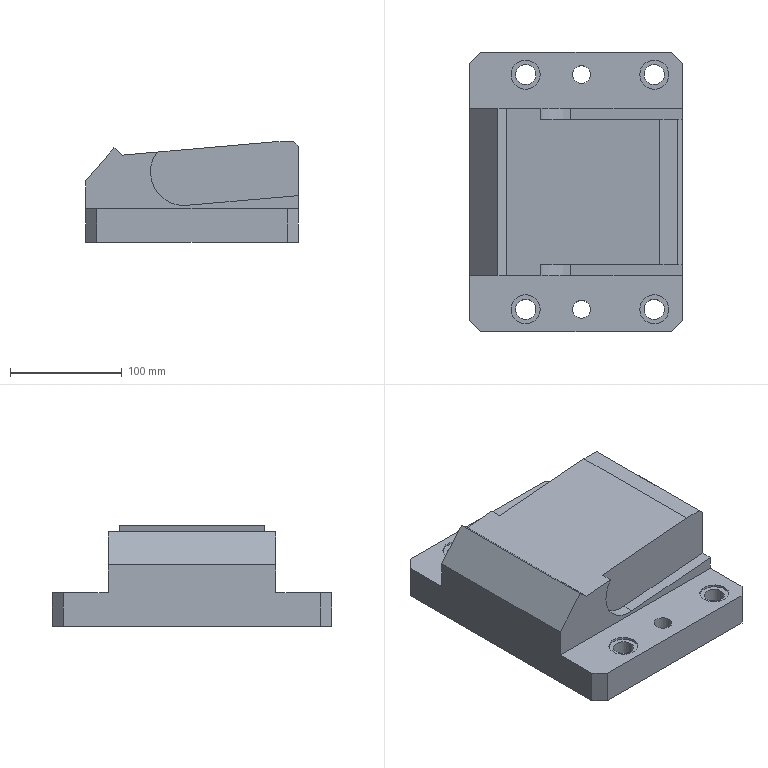Part | NX | features solid 2 | 1 solid | 51 faces | box 190 x 250 x 90 mm | volume 2700369 mm3 | plane 35 | cylinder 16 | commonest cylinder face diameters 18 x4 20 x4 26 x4 16 x2 60 x2
STEP:
#1=CARTESIAN_POINT('',(1060.,115.,-248.228));
#2=VERTEX_POINT('',#1);
#3=CARTESIAN_POINT('',(1060.,115.,-204.));
#4=VERTEX_POINT('',#3);
#5=CARTESIAN_POINT('',(1060.,115.,-218.327));
#6=DIRECTION('',(0.,0.,1.));
#7=VECTOR('',#6,1000.);
#8=LINE('',#5,#7);
#9=EDGE_CURVE('',#2,#4,#8,.T.);
#10=ORIENTED_EDGE('',*,*,#9,.F.);
#11=CARTESIAN_POINT('',(1060.,105.,-248.228));
#12=VERTEX_POINT('',#11);
#13=CARTESIAN_POINT('',(1060.,180.,-248.228));
#14=DIRECTION('',(0.,-1.,0.));
#15=VECTOR('',#14,1000.);
#16=LINE('',#13,#15);
#17=EDGE_CURVE('',#12,#2,#16,.F.);
#18=ORIENTED_EDGE('',*,*,#17,.F.);
#19=CARTESIAN_POINT('',(1060.,105.,-260.));
#20=VERTEX_POINT('',#19);
#21=CARTESIAN_POINT('',(1060.,105.,-200.));
#22=DIRECTION('',(0.,0.,-1.));
#23=VECTOR('',#22,1000.);
#24=LINE('',#21,#23);
#25=EDGE_CURVE('',#12,#20,#24,.T.);
#26=ORIENTED_EDGE('',*,*,#25,.T.);
#27=CARTESIAN_POINT('',(1060.,65.,-260.));
#28=VERTEX_POINT('',#27);
#29=CARTESIAN_POINT('',(1060.,305.,-260.));
#30=DIRECTION('',(0.,-1.,0.));
#31=VECTOR('',#30,1000.);
#32=LINE('',#29,#31);
#33=EDGE_CURVE('',#20,#28,#32,.T.);
#34=ORIENTED_EDGE('',*,*,#33,.T.);
#35=CARTESIAN_POINT('',(1060.,65.,-290.));
#36=VERTEX_POINT('',#35);
#37=CARTESIAN_POINT('',(1060.,65.,-260.));
#38=DIRECTION('',(0.,0.,1.));
#39=VECTOR('',#38,1000.);
#40=LINE('',#37,#39);
#41=EDGE_CURVE('',#36,#28,#40,.T.);
#42=ORIENTED_EDGE('',*,*,#41,.F.);
#43=CARTESIAN_POINT('',(1060.,295.,-290.));
#44=VERTEX_POINT('',#43);
#45=CARTESIAN_POINT('',(1060.,305.,-290.));
#46=DIRECTION('',(0.,-1.,0.));
#47=VECTOR('',#46,1000.);
#48=LINE('',#45,#47);
#49=EDGE_CURVE('',#44,#36,#48,.T.);
#50=ORIENTED_EDGE('',*,*,#49,.F.);
#51=CARTESIAN_POINT('',(1060.,295.,-260.));
#52=VERTEX_POINT('',#51);
#53=CARTESIAN_POINT('',(1060.,295.,-260.));
#54=DIRECTION('',(0.,0.,-1.));
#55=VECTOR('',#54,1000.);
#56=LINE('',#53,#55);
#57=EDGE_CURVE('',#52,#44,#56,.T.);
#58=ORIENTED_EDGE('',*,*,#57,.F.);
#59=CARTESIAN_POINT('',(1060.,255.,-260.));
#60=VERTEX_POINT('',#59);
#61=CARTESIAN_POINT('',(1060.,305.,-260.));
#62=DIRECTION('',(0.,-1.,0.));
#63=VECTOR('',#62,1000.);
#64=LINE('',#61,#63);
#65=EDGE_CURVE('',#52,#60,#64,.T.);
#66=ORIENTED_EDGE('',*,*,#65,.T.);
#67=CARTESIAN_POINT('',(1060.,255.,-248.228));
#68=VERTEX_POINT('',#67);
#69=CARTESIAN_POINT('',(1060.,255.,-200.));
#70=DIRECTION('',(0.,0.,-1.));
#71=VECTOR('',#70,1000.);
#72=LINE('',#69,#71);
#73=EDGE_CURVE('',#68,#60,#72,.T.);
#74=ORIENTED_EDGE('',*,*,#73,.F.);
#75=CARTESIAN_POINT('',(1060.,245.,-248.228));
#76=VERTEX_POINT('',#75);
#77=CARTESIAN_POINT('',(1060.,180.,-248.228));
#78=DIRECTION('',(0.,1.,0.));
#79=VECTOR('',#78,1000.);
#80=LINE('',#77,#79);
#81=EDGE_CURVE('',#68,#76,#80,.F.);
#82=ORIENTED_EDGE('',*,*,#81,.T.);
#83=CARTESIAN_POINT('',(1060.,245.,-204.));
#84=VERTEX_POINT('',#83);
#85=CARTESIAN_POINT('',(1060.,245.,-218.327));
#86=DIRECTION('',(0.,0.,1.));
#87=VECTOR('',#86,1000.);
#88=LINE('',#85,#87);
#89=EDGE_CURVE('',#76,#84,#88,.T.);
#90=ORIENTED_EDGE('',*,*,#89,.T.);
#91=CARTESIAN_POINT('',(1060.,305.,-204.));
#92=DIRECTION('',(0.,1.,0.));
#93=VECTOR('',#92,1000.);
#94=LINE('',#91,#93);
#95=EDGE_CURVE('',#4,#84,#94,.T.);
#96=ORIENTED_EDGE('',*,*,#95,.F.);
#97=EDGE_LOOP('',(#10,#18,#26,#34,#42,#50,#58,#66,#74,#82,#90,#96));
#98=FACE_BOUND('',#97,.T.);
#99=CARTESIAN_POINT('',(1060.,305.,-260.));
#100=DIRECTION('',(1.,0.,0.));
#101=DIRECTION('',(0.,-1.,0.));
#102=AXIS2_PLACEMENT_3D('',#99,#100,#101);
#103=PLANE('',#102);
#104=ADVANCED_FACE('',(#98),#103,.T.);
#105=CARTESIAN_POINT('',(933.612,245.,-209.308));
#106=VERTEX_POINT('',#105);
#107=CARTESIAN_POINT('',(933.612,255.,-209.308));
#108=VERTEX_POINT('',#107);
#109=CARTESIAN_POINT('',(933.612,250.,-209.308));
#110=DIRECTION('',(0.,1.,0.));
#111=VECTOR('',#110,1000.);
#112=LINE('',#109,#111);
#113=EDGE_CURVE('',#106,#108,#112,.T.);
#114=ORIENTED_EDGE('',*,*,#113,.T.);
#115=CARTESIAN_POINT('',(902.806,255.,-212.003));
#116=VERTEX_POINT('',#115);
#117=CARTESIAN_POINT('',(1040.,255.,-200.));
#118=DIRECTION('',(-0.9962,0.,-0.08716));
#119=VECTOR('',#118,1000.);
#120=LINE('',#117,#119);
#121=EDGE_CURVE('',#108,#116,#120,.T.);
#122=ORIENTED_EDGE('',*,*,#121,.T.);
#123=CARTESIAN_POINT('',(902.806,105.,-212.003));
#124=VERTEX_POINT('',#123);
#125=CARTESIAN_POINT('',(902.806,255.,-212.003));
#126=DIRECTION('',(0.,-1.,0.));
#127=VECTOR('',#126,1000.);
#128=LINE('',#125,#127);
#129=EDGE_CURVE('',#116,#124,#128,.T.);
#130=ORIENTED_EDGE('',*,*,#129,.T.);
#131=CARTESIAN_POINT('',(933.612,105.,-209.308));
#132=VERTEX_POINT('',#131);
#133=CARTESIAN_POINT('',(1040.,105.,-200.));
#134=DIRECTION('',(-0.9962,0.,-0.08716));
#135=VECTOR('',#134,1000.);
#136=LINE('',#133,#135);
#137=EDGE_CURVE('',#132,#124,#136,.T.);
#138=ORIENTED_EDGE('',*,*,#137,.F.);
#139=CARTESIAN_POINT('',(933.612,115.,-209.308));
#140=VERTEX_POINT('',#139);
#141=CARTESIAN_POINT('',(933.612,110.,-209.308));
#142=DIRECTION('',(0.,1.,0.));
#143=VECTOR('',#142,1000.);
#144=LINE('',#141,#143);
#145=EDGE_CURVE('',#132,#140,#144,.T.);
#146=ORIENTED_EDGE('',*,*,#145,.T.);
#147=CARTESIAN_POINT('',(1040.,115.,-200.));
#148=VERTEX_POINT('',#147);
#149=CARTESIAN_POINT('',(1040.,115.,-200.));
#150=DIRECTION('',(0.9962,0.,0.08716));
#151=VECTOR('',#150,1000.);
#152=LINE('',#149,#151);
#153=EDGE_CURVE('',#140,#148,#152,.T.);
#154=ORIENTED_EDGE('',*,*,#153,.T.);
#155=CARTESIAN_POINT('',(1040.,245.,-200.));
#156=VERTEX_POINT('',#155);
#157=CARTESIAN_POINT('',(1040.,255.,-200.));
#158=DIRECTION('',(0.,-1.,0.));
#159=VECTOR('',#158,1000.);
#160=LINE('',#157,#159);
#161=EDGE_CURVE('',#156,#148,#160,.T.);
#162=ORIENTED_EDGE('',*,*,#161,.F.);
#163=CARTESIAN_POINT('',(1040.,245.,-200.));
#164=DIRECTION('',(-0.9962,0.,-0.08716));
#165=VECTOR('',#164,1000.);
#166=LINE('',#163,#165);
#167=EDGE_CURVE('',#156,#106,#166,.T.);
#168=ORIENTED_EDGE('',*,*,#167,.T.);
#169=EDGE_LOOP('',(#114,#122,#130,#138,#146,#154,#162,#168));
#170=FACE_BOUND('',#169,.T.);
#171=CARTESIAN_POINT('',(1040.,255.,-200.));
#172=DIRECTION('',(0.08716,0.,-0.9962));
#173=DIRECTION('',(-0.9962,0.,-0.08716));
#174=AXIS2_PLACEMENT_3D('',#171,#172,#173);
#175=PLANE('',#174);
#176=ADVANCED_FACE('',(#170),#175,.F.);
#177=CARTESIAN_POINT('',(1056.,245.,-200.));
#178=VERTEX_POINT('',#177);
#179=CARTESIAN_POINT('',(1040.,245.,-200.));
#180=DIRECTION('',(1.,0.,0.));
#181=VECTOR('',#180,1000.);
#182=LINE('',#179,#181);
#183=EDGE_CURVE('',#156,#178,#182,.T.);
#184=ORIENTED_EDGE('',*,*,#183,.F.);
#185=ORIENTED_EDGE('',*,*,#161,.T.);
#186=CARTESIAN_POINT('',(1056.,115.,-200.));
#187=VERTEX_POINT('',#186);
#188=CARTESIAN_POINT('',(1040.,115.,-200.));
#189=DIRECTION('',(-1.,0.,0.));
#190=VECTOR('',#189,1000.);
#191=LINE('',#188,#190);
#192=EDGE_CURVE('',#187,#148,#191,.T.);
#193=ORIENTED_EDGE('',*,*,#192,.F.);
#194=CARTESIAN_POINT('',(1056.,255.,-200.));
#195=DIRECTION('',(0.,-1.,0.));
#196=VECTOR('',#195,1000.);
#197=LINE('',#194,#196);
#198=EDGE_CURVE('',#178,#187,#197,.T.);
#199=ORIENTED_EDGE('',*,*,#198,.F.);
#200=EDGE_LOOP('',(#184,#185,#193,#199));
#201=FACE_BOUND('',#200,.T.);
#202=CARTESIAN_POINT('',(1040.,255.,-200.));
#203=DIRECTION('',(0.,0.,1.));
#204=DIRECTION('',(0.,-1.,0.));
#205=AXIS2_PLACEMENT_3D('',#202,#203,#204);
#206=PLANE('',#205);
#207=ADVANCED_FACE('',(#201),#206,.T.);
#208=ORIENTED_EDGE('',*,*,#73,.T.);
#209=CARTESIAN_POINT('',(870.,255.,-260.));
#210=VERTEX_POINT('',#209);
#211=CARTESIAN_POINT('',(870.,255.,-260.));
#212=DIRECTION('',(1.,0.,0.));
#213=VECTOR('',#212,1000.);
#214=LINE('',#211,#213);
#215=EDGE_CURVE('',#210,#60,#214,.T.);
#216=ORIENTED_EDGE('',*,*,#215,.F.);
#217=CARTESIAN_POINT('',(870.,255.,-235.));
#218=VERTEX_POINT('',#217);
#219=CARTESIAN_POINT('',(870.,255.,-235.));
#220=DIRECTION('',(0.,0.,-1.));
#221=VECTOR('',#220,1000.);
#222=LINE('',#219,#221);
#223=EDGE_CURVE('',#218,#210,#222,.T.);
#224=ORIENTED_EDGE('',*,*,#223,.F.);
#225=CARTESIAN_POINT('',(895.204,255.,-205.506));
#226=VERTEX_POINT('',#225);
#227=CARTESIAN_POINT('',(870.,255.,-235.));
#228=DIRECTION('',(0.6497,0.,0.7602));
#229=VECTOR('',#228,1000.);
#230=LINE('',#227,#229);
#231=EDGE_CURVE('',#218,#226,#230,.T.);
#232=ORIENTED_EDGE('',*,*,#231,.T.);
#233=CARTESIAN_POINT('',(895.204,255.,-205.506));
#234=DIRECTION('',(0.7602,0.,-0.6497));
#235=VECTOR('',#234,1000.);
#236=LINE('',#233,#235);
#237=EDGE_CURVE('',#226,#116,#236,.T.);
#238=ORIENTED_EDGE('',*,*,#237,.T.);
#239=ORIENTED_EDGE('',*,*,#121,.F.);
#240=CARTESIAN_POINT('',(960.414,255.,-256.94));
#241=VERTEX_POINT('',#240);
#242=CARTESIAN_POINT('',(957.8,255.,-227.054));
#243=DIRECTION('',(0.,-1.,0.));
#244=DIRECTION('',(1.,0.,0.));
#245=AXIS2_PLACEMENT_3D('',#242,#243,#244);
#246=CIRCLE('',#245,30.);
#247=EDGE_CURVE('',#241,#108,#246,.F.);
#248=ORIENTED_EDGE('',*,*,#247,.F.);
#249=CARTESIAN_POINT('',(1060.,255.,-248.228));
#250=DIRECTION('',(-0.9962,0.,-0.08716));
#251=VECTOR('',#250,1000.);
#252=LINE('',#249,#251);
#253=EDGE_CURVE('',#68,#241,#252,.T.);
#254=ORIENTED_EDGE('',*,*,#253,.F.);
#255=EDGE_LOOP('',(#208,#216,#224,#232,#238,#239,#248,#254));
#256=FACE_BOUND('',#255,.T.);
#257=CARTESIAN_POINT('',(870.,255.,-214.873));
#258=DIRECTION('',(0.,1.,0.));
#259=DIRECTION('',(1.,0.,0.));
#260=AXIS2_PLACEMENT_3D('',#257,#258,#259);
#261=PLANE('',#260);
#262=ADVANCED_FACE('',(#256),#261,.T.);
#263=CARTESIAN_POINT('',(960.414,105.,-256.94));
#264=VERTEX_POINT('',#263);
#265=CARTESIAN_POINT('',(1060.,105.,-248.228));
#266=DIRECTION('',(-0.9962,0.,-0.08716));
#267=VECTOR('',#266,1000.);
#268=LINE('',#265,#267);
#269=EDGE_CURVE('',#12,#264,#268,.T.);
#270=ORIENTED_EDGE('',*,*,#269,.T.);
#271=CARTESIAN_POINT('',(957.8,105.,-227.054));
#272=DIRECTION('',(0.,-1.,0.));
#273=DIRECTION('',(1.,0.,0.));
#274=AXIS2_PLACEMENT_3D('',#271,#272,#273);
#275=CIRCLE('',#274,30.);
#276=EDGE_CURVE('',#132,#264,#275,.T.);
#277=ORIENTED_EDGE('',*,*,#276,.F.);
#278=ORIENTED_EDGE('',*,*,#137,.T.);
#279=CARTESIAN_POINT('',(895.204,105.,-205.506));
#280=VERTEX_POINT('',#279);
#281=CARTESIAN_POINT('',(895.204,105.,-205.506));
#282=DIRECTION('',(0.7602,0.,-0.6497));
#283=VECTOR('',#282,1000.);
#284=LINE('',#281,#283);
#285=EDGE_CURVE('',#280,#124,#284,.T.);
#286=ORIENTED_EDGE('',*,*,#285,.F.);
#287=CARTESIAN_POINT('',(870.,105.,-235.));
#288=VERTEX_POINT('',#287);
#289=CARTESIAN_POINT('',(870.,105.,-235.));
#290=DIRECTION('',(0.6497,0.,0.7602));
#291=VECTOR('',#290,1000.);
#292=LINE('',#289,#291);
#293=EDGE_CURVE('',#288,#280,#292,.T.);
#294=ORIENTED_EDGE('',*,*,#293,.F.);
#295=CARTESIAN_POINT('',(870.,105.,-260.));
#296=VERTEX_POINT('',#295);
#297=CARTESIAN_POINT('',(870.,105.,-235.));
#298=DIRECTION('',(0.,0.,-1.));
#299=VECTOR('',#298,1000.);
#300=LINE('',#297,#299);
#301=EDGE_CURVE('',#288,#296,#300,.T.);
#302=ORIENTED_EDGE('',*,*,#301,.T.);
#303=CARTESIAN_POINT('',(870.,105.,-260.));
#304=DIRECTION('',(1.,0.,0.));
#305=VECTOR('',#304,1000.);
#306=LINE('',#303,#305);
#307=EDGE_CURVE('',#296,#20,#306,.T.);
#308=ORIENTED_EDGE('',*,*,#307,.T.);
#309=ORIENTED_EDGE('',*,*,#25,.F.);
#310=EDGE_LOOP('',(#270,#277,#278,#286,#294,#302,#308,#309));
#311=FACE_BOUND('',#310,.T.);
#312=CARTESIAN_POINT('',(870.,105.,-214.873));
#313=DIRECTION('',(0.,1.,0.));
#314=DIRECTION('',(1.,0.,0.));
#315=AXIS2_PLACEMENT_3D('',#312,#313,#314);
#316=PLANE('',#315);
#317=ADVANCED_FACE('',(#311),#316,.F.);
#318=CARTESIAN_POINT('',(978.,75.,-260.));
#319=VERTEX_POINT('',#318);
#320=CARTESIAN_POINT('',(970.,75.,-260.));
#321=DIRECTION('',(0.,0.,1.));
#322=DIRECTION('',(1.,0.,0.));
#323=AXIS2_PLACEMENT_3D('',#320,#321,#322);
#324=CIRCLE('',#323,8.);
#325=EDGE_CURVE('',#319,#319,#324,.T.);
#326=ORIENTED_EDGE('',*,*,#325,.F.);
#327=EDGE_LOOP('',(#326));
#328=FACE_BOUND('',#327,.T.);
#329=CARTESIAN_POINT('',(907.,75.,-260.));
#330=VERTEX_POINT('',#329);
#331=CARTESIAN_POINT('',(920.,75.,-260.));
#332=DIRECTION('',(0.,0.,-1.));
#333=DIRECTION('',(-1.,0.,0.));
#334=AXIS2_PLACEMENT_3D('',#331,#332,#333);
#335=CIRCLE('',#334,13.);
#336=EDGE_CURVE('',#330,#330,#335,.F.);
#337=ORIENTED_EDGE('',*,*,#336,.F.);
#338=EDGE_LOOP('',(#337));
#339=FACE_BOUND('',#338,.T.);
#340=CARTESIAN_POINT('',(1022.,75.,-260.));
#341=VERTEX_POINT('',#340);
#342=CARTESIAN_POINT('',(1035.,75.,-260.));
#343=DIRECTION('',(0.,0.,-1.));
#344=DIRECTION('',(-1.,0.,0.));
#345=AXIS2_PLACEMENT_3D('',#342,#343,#344);
#346=CIRCLE('',#345,13.);
#347=EDGE_CURVE('',#341,#341,#346,.F.);
#348=ORIENTED_EDGE('',*,*,#347,.F.);
#349=EDGE_LOOP('',(#348));
#350=FACE_BOUND('',#349,.T.);
#351=CARTESIAN_POINT('',(880.,55.,-260.));
#352=VERTEX_POINT('',#351);
#353=CARTESIAN_POINT('',(1050.,55.,-260.));
#354=VERTEX_POINT('',#353);
#355=CARTESIAN_POINT('',(870.,55.,-260.));
#356=DIRECTION('',(1.,0.,0.));
#357=VECTOR('',#356,1000.);
#358=LINE('',#355,#357);
#359=EDGE_CURVE('',#352,#354,#358,.T.);
#360=ORIENTED_EDGE('',*,*,#359,.T.);
#361=CARTESIAN_POINT('',(1085.,90.,-260.));
#362=DIRECTION('',(-0.7071,-0.7071,0.));
#363=VECTOR('',#362,1000.);
#364=LINE('',#361,#363);
#365=EDGE_CURVE('',#28,#354,#364,.T.);
#366=ORIENTED_EDGE('',*,*,#365,.F.);
#367=ORIENTED_EDGE('',*,*,#33,.F.);
#368=ORIENTED_EDGE('',*,*,#307,.F.);
#369=CARTESIAN_POINT('',(870.,65.,-260.));
#370=VERTEX_POINT('',#369);
#371=CARTESIAN_POINT('',(870.,305.,-260.));
#372=DIRECTION('',(0.,-1.,0.));
#373=VECTOR('',#372,1000.);
#374=LINE('',#371,#373);
#375=EDGE_CURVE('',#296,#370,#374,.T.);
#376=ORIENTED_EDGE('',*,*,#375,.T.);
#377=CARTESIAN_POINT('',(750.,185.,-260.));
#378=DIRECTION('',(0.7071,-0.7071,0.));
#379=VECTOR('',#378,1000.);
#380=LINE('',#377,#379);
#381=EDGE_CURVE('',#352,#370,#380,.F.);
#382=ORIENTED_EDGE('',*,*,#381,.F.);
#383=EDGE_LOOP('',(#360,#366,#367,#368,#376,#382));
#384=FACE_BOUND('',#383,.T.);
#385=CARTESIAN_POINT('',(870.,305.,-260.));
#386=DIRECTION('',(0.,0.,1.));
#387=DIRECTION('',(1.,0.,0.));
#388=AXIS2_PLACEMENT_3D('',#385,#386,#387);
#389=PLANE('',#388);
#390=ADVANCED_FACE('',(#328,#339,#350,#384),#389,.T.);
#391=CARTESIAN_POINT('',(870.,295.,-290.));
#392=VERTEX_POINT('',#391);
#393=CARTESIAN_POINT('',(870.,65.,-290.));
#394=VERTEX_POINT('',#393);
#395=CARTESIAN_POINT('',(870.,305.,-290.));
#396=DIRECTION('',(0.,-1.,0.));
#397=VECTOR('',#396,1000.);
#398=LINE('',#395,#397);
#399=EDGE_CURVE('',#392,#394,#398,.T.);
#400=ORIENTED_EDGE('',*,*,#399,.T.);
#401=CARTESIAN_POINT('',(870.,65.,-260.));
#402=DIRECTION('',(0.,0.,-1.));
#403=VECTOR('',#402,1000.);
#404=LINE('',#401,#403);
#405=EDGE_CURVE('',#370,#394,#404,.T.);
#406=ORIENTED_EDGE('',*,*,#405,.F.);
#407=ORIENTED_EDGE('',*,*,#375,.F.);
#408=ORIENTED_EDGE('',*,*,#301,.F.);
#409=CARTESIAN_POINT('',(870.,255.,-235.));
#410=DIRECTION('',(0.,-1.,0.));
#411=VECTOR('',#410,1000.);
#412=LINE('',#409,#411);
#413=EDGE_CURVE('',#218,#288,#412,.T.);
#414=ORIENTED_EDGE('',*,*,#413,.F.);
#415=ORIENTED_EDGE('',*,*,#223,.T.);
#416=CARTESIAN_POINT('',(870.,295.,-260.));
#417=VERTEX_POINT('',#416);
#418=CARTESIAN_POINT('',(870.,305.,-260.));
#419=DIRECTION('',(0.,-1.,0.));
#420=VECTOR('',#419,1000.);
#421=LINE('',#418,#420);
#422=EDGE_CURVE('',#417,#210,#421,.T.);
#423=ORIENTED_EDGE('',*,*,#422,.F.);
#424=CARTESIAN_POINT('',(870.,295.,-260.));
#425=DIRECTION('',(0.,0.,1.));
#426=VECTOR('',#425,1000.);
#427=LINE('',#424,#426);
#428=EDGE_CURVE('',#392,#417,#427,.T.);
#429=ORIENTED_EDGE('',*,*,#428,.F.);
#430=EDGE_LOOP('',(#400,#406,#407,#408,#414,#415,#423,#429));
#431=FACE_BOUND('',#430,.T.);
#432=CARTESIAN_POINT('',(870.,305.,-260.));
#433=DIRECTION('',(1.,0.,0.));
#434=DIRECTION('',(0.,-1.,0.));
#435=AXIS2_PLACEMENT_3D('',#432,#433,#434);
#436=PLANE('',#435);
#437=ADVANCED_FACE('',(#431),#436,.F.);
#438=CARTESIAN_POINT('',(978.,75.,-290.));
#439=VERTEX_POINT('',#438);
#440=CARTESIAN_POINT('',(970.,75.,-290.));
#441=DIRECTION('',(0.,0.,1.));
#442=DIRECTION('',(1.,0.,0.));
#443=AXIS2_PLACEMENT_3D('',#440,#441,#442);
#444=CIRCLE('',#443,8.);
#445=EDGE_CURVE('',#439,#439,#444,.T.);
#446=ORIENTED_EDGE('',*,*,#445,.T.);
#447=EDGE_LOOP('',(#446));
#448=FACE_BOUND('',#447,.T.);
#449=CARTESIAN_POINT('',(978.,285.,-290.));
#450=VERTEX_POINT('',#449);
#451=CARTESIAN_POINT('',(970.,285.,-290.));
#452=DIRECTION('',(0.,0.,1.));
#453=DIRECTION('',(1.,0.,0.));
#454=AXIS2_PLACEMENT_3D('',#451,#452,#453);
#455=CIRCLE('',#454,8.);
#456=EDGE_CURVE('',#450,#450,#455,.T.);
#457=ORIENTED_EDGE('',*,*,#456,.T.);
#458=EDGE_LOOP('',(#457));
#459=FACE_BOUND('',#458,.T.);
#460=CARTESIAN_POINT('',(995.,196.,-290.));
#461=VERTEX_POINT('',#460);
#462=CARTESIAN_POINT('',(945.,196.,-290.));
#463=VERTEX_POINT('',#462);
#464=CARTESIAN_POINT('',(995.,196.,-290.));
#465=DIRECTION('',(-1.,0.,0.));
#466=VECTOR('',#465,1000.);
#467=LINE('',#464,#466);
#468=EDGE_CURVE('',#461,#463,#467,.T.);
#469=ORIENTED_EDGE('',*,*,#468,.T.);
#470=CARTESIAN_POINT('',(945.,220.,-290.));
#471=VERTEX_POINT('',#470);
#472=CARTESIAN_POINT('',(945.,180.,-290.));
#473=DIRECTION('',(0.,-1.,0.));
#474=VECTOR('',#473,1000.);
#475=LINE('',#472,#474);
#476=EDGE_CURVE('',#471,#463,#475,.T.);
#477=ORIENTED_EDGE('',*,*,#476,.F.);
#478=CARTESIAN_POINT('',(925.,220.,-290.));
#479=VERTEX_POINT('',#478);
#480=CARTESIAN_POINT('',(935.,220.,-290.));
#481=DIRECTION('',(0.,0.,1.));
#482=DIRECTION('',(-1.,0.,0.));
#483=AXIS2_PLACEMENT_3D('',#480,#481,#482);
#484=CIRCLE('',#483,10.);
#485=EDGE_CURVE('',#471,#479,#484,.T.);
#486=ORIENTED_EDGE('',*,*,#485,.T.);
#487=CARTESIAN_POINT('',(925.,140.,-290.));
#488=VERTEX_POINT('',#487);
#489=CARTESIAN_POINT('',(925.,180.,-290.));
#490=DIRECTION('',(0.,-1.,0.));
#491=VECTOR('',#490,1000.);
#492=LINE('',#489,#491);
#493=EDGE_CURVE('',#479,#488,#492,.T.);
#494=ORIENTED_EDGE('',*,*,#493,.T.);
#495=CARTESIAN_POINT('',(945.,140.,-290.));
#496=VERTEX_POINT('',#495);
#497=CARTESIAN_POINT('',(935.,140.,-290.));
#498=DIRECTION('',(0.,0.,1.));
#499=DIRECTION('',(-1.,0.,0.));
#500=AXIS2_PLACEMENT_3D('',#497,#498,#499);
#501=CIRCLE('',#500,10.);
#502=EDGE_CURVE('',#488,#496,#501,.T.);
#503=ORIENTED_EDGE('',*,*,#502,.T.);
#504=CARTESIAN_POINT('',(945.,164.,-290.));
#505=VERTEX_POINT('',#504);
#506=CARTESIAN_POINT('',(945.,180.,-290.));
#507=DIRECTION('',(0.,-1.,0.));
#508=VECTOR('',#507,1000.);
#509=LINE('',#506,#508);
#510=EDGE_CURVE('',#505,#496,#509,.T.);
#511=ORIENTED_EDGE('',*,*,#510,.F.);
#512=CARTESIAN_POINT('',(995.,164.,-290.));
#513=VERTEX_POINT('',#512);
#514=CARTESIAN_POINT('',(995.,164.,-290.));
#515=DIRECTION('',(-1.,0.,0.));
#516=VECTOR('',#515,1000.);
#517=LINE('',#514,#516);
#518=EDGE_CURVE('',#513,#505,#517,.T.);
#519=ORIENTED_EDGE('',*,*,#518,.F.);
#520=CARTESIAN_POINT('',(995.,140.,-290.));
#521=VERTEX_POINT('',#520);
#522=CARTESIAN_POINT('',(995.,180.,-290.));
#523=DIRECTION('',(0.,-1.,0.));
#524=VECTOR('',#523,1000.);
#525=LINE('',#522,#524);
#526=EDGE_CURVE('',#513,#521,#525,.T.);
#527=ORIENTED_EDGE('',*,*,#526,.T.);
#528=CARTESIAN_POINT('',(1015.,140.,-290.));
#529=VERTEX_POINT('',#528);
#530=CARTESIAN_POINT('',(1005.,140.,-290.));
#531=DIRECTION('',(0.,0.,1.));
#532=DIRECTION('',(-1.,0.,0.));
#533=AXIS2_PLACEMENT_3D('',#530,#531,#532);
#534=CIRCLE('',#533,10.);
#535=EDGE_CURVE('',#521,#529,#534,.T.);
#536=ORIENTED_EDGE('',*,*,#535,.T.);
#537=CARTESIAN_POINT('',(1015.,220.,-290.));
#538=VERTEX_POINT('',#537);
#539=CARTESIAN_POINT('',(1015.,180.,-290.));
#540=DIRECTION('',(0.,-1.,0.));
#541=VECTOR('',#540,1000.);
#542=LINE('',#539,#541);
#543=EDGE_CURVE('',#538,#529,#542,.T.);
#544=ORIENTED_EDGE('',*,*,#543,.F.);
#545=CARTESIAN_POINT('',(995.,220.,-290.));
#546=VERTEX_POINT('',#545);
#547=CARTESIAN_POINT('',(1005.,220.,-290.));
#548=DIRECTION('',(0.,0.,1.));
#549=DIRECTION('',(-1.,0.,0.));
#550=AXIS2_PLACEMENT_3D('',#547,#548,#549);
#551=CIRCLE('',#550,10.);
#552=EDGE_CURVE('',#538,#546,#551,.T.);
#553=ORIENTED_EDGE('',*,*,#552,.T.);
#554=CARTESIAN_POINT('',(995.,180.,-290.));
#555=DIRECTION('',(0.,-1.,0.));
#556=VECTOR('',#555,1000.);
#557=LINE('',#554,#556);
#558=EDGE_CURVE('',#546,#461,#557,.T.);
#559=ORIENTED_EDGE('',*,*,#558,.T.);
#560=EDGE_LOOP('',(#469,#477,#486,#494,#503,#511,#519,#527,#536,#544,#553,#559));
#561=FACE_BOUND('',#560,.T.);
#562=CARTESIAN_POINT('',(929.,285.,-290.));
#563=VERTEX_POINT('',#562);
#564=CARTESIAN_POINT('',(920.,285.,-290.));
#565=DIRECTION('',(0.,0.,1.));
#566=DIRECTION('',(1.,0.,0.));
#567=AXIS2_PLACEMENT_3D('',#564,#565,#566);
#568=CIRCLE('',#567,9.);
#569=EDGE_CURVE('',#563,#563,#568,.T.);
#570=ORIENTED_EDGE('',*,*,#569,.T.);
#571=EDGE_LOOP('',(#570));
#572=FACE_BOUND('',#571,.T.);
#573=CARTESIAN_POINT('',(1044.,285.,-290.));
#574=VERTEX_POINT('',#573);
#575=CARTESIAN_POINT('',(1035.,285.,-290.));
#576=DIRECTION('',(0.,0.,1.));
#577=DIRECTION('',(1.,0.,0.));
#578=AXIS2_PLACEMENT_3D('',#575,#576,#577);
#579=CIRCLE('',#578,9.);
#580=EDGE_CURVE('',#574,#574,#579,.T.);
#581=ORIENTED_EDGE('',*,*,#580,.T.);
#582=EDGE_LOOP('',(#581));
#583=FACE_BOUND('',#582,.T.);
#584=CARTESIAN_POINT('',(929.,75.,-290.));
#585=VERTEX_POINT('',#584);
#586=CARTESIAN_POINT('',(920.,75.,-290.));
#587=DIRECTION('',(0.,0.,1.));
#588=DIRECTION('',(1.,0.,0.));
#589=AXIS2_PLACEMENT_3D('',#586,#587,#588);
#590=CIRCLE('',#589,9.);
#591=EDGE_CURVE('',#585,#585,#590,.T.);
#592=ORIENTED_EDGE('',*,*,#591,.T.);
#593=EDGE_LOOP('',(#592));
#594=FACE_BOUND('',#593,.T.);
#595=CARTESIAN_POINT('',(1044.,75.,-290.));
#596=VERTEX_POINT('',#595);
#597=CARTESIAN_POINT('',(1035.,75.,-290.));
#598=DIRECTION('',(0.,0.,1.));
#599=DIRECTION('',(1.,0.,0.));
#600=AXIS2_PLACEMENT_3D('',#597,#598,#599);
#601=CIRCLE('',#600,9.);
#602=EDGE_CURVE('',#596,#596,#601,.T.);
#603=ORIENTED_EDGE('',*,*,#602,.T.);
#604=EDGE_LOOP('',(#603));
#605=FACE_BOUND('',#604,.T.);
#606=ORIENTED_EDGE('',*,*,#49,.T.);
#607=CARTESIAN_POINT('',(1050.,55.,-290.));
#608=VERTEX_POINT('',#607);
#609=CARTESIAN_POINT('',(1180.,185.,-290.));
#610=DIRECTION('',(0.7071,0.7071,0.));
#611=VECTOR('',#610,1000.);
#612=LINE('',#609,#611);
#613=EDGE_CURVE('',#608,#36,#612,.T.);
#614=ORIENTED_EDGE('',*,*,#613,.F.);
#615=CARTESIAN_POINT('',(880.,55.,-290.));
#616=VERTEX_POINT('',#615);
#617=CARTESIAN_POINT('',(1060.,55.,-290.));
#618=DIRECTION('',(-1.,0.,0.));
#619=VECTOR('',#618,1000.);
#620=LINE('',#617,#619);
#621=EDGE_CURVE('',#608,#616,#620,.T.);
#622=ORIENTED_EDGE('',*,*,#621,.T.);
#623=CARTESIAN_POINT('',(845.,90.,-290.));
#624=DIRECTION('',(-0.7071,0.7071,0.));
#625=VECTOR('',#624,1000.);
#626=LINE('',#623,#625);
#627=EDGE_CURVE('',#394,#616,#626,.F.);
#628=ORIENTED_EDGE('',*,*,#627,.F.);
#629=ORIENTED_EDGE('',*,*,#399,.F.);
#630=CARTESIAN_POINT('',(880.,305.,-290.));
#631=VERTEX_POINT('',#630);
#632=CARTESIAN_POINT('',(970.,395.,-290.));
#633=DIRECTION('',(-0.7071,-0.7071,0.));
#634=VECTOR('',#633,1000.);
#635=LINE('',#632,#634);
#636=EDGE_CURVE('',#631,#392,#635,.T.);
#637=ORIENTED_EDGE('',*,*,#636,.F.);
#638=CARTESIAN_POINT('',(1050.,305.,-290.));
#639=VERTEX_POINT('',#638);
#640=CARTESIAN_POINT('',(1060.,305.,-290.));
#641=DIRECTION('',(-1.,0.,0.));
#642=VECTOR('',#641,1000.);
#643=LINE('',#640,#642);
#644=EDGE_CURVE('',#639,#631,#643,.T.);
#645=ORIENTED_EDGE('',*,*,#644,.F.);
#646=CARTESIAN_POINT('',(1055.,300.,-290.));
#647=DIRECTION('',(0.7071,-0.7071,0.));
#648=VECTOR('',#647,1000.);
#649=LINE('',#646,#648);
#650=EDGE_CURVE('',#44,#639,#649,.F.);
#651=ORIENTED_EDGE('',*,*,#650,.F.);
#652=EDGE_LOOP('',(#606,#614,#622,#628,#629,#637,#645,#651));
#653=FACE_BOUND('',#652,.T.);
#654=CARTESIAN_POINT('',(1060.,305.,-290.));
#655=DIRECTION('',(0.,0.,-1.));
#656=DIRECTION('',(-1.,0.,0.));
#657=AXIS2_PLACEMENT_3D('',#654,#655,#656);
#658=PLANE('',#657);
#659=ADVANCED_FACE('',(#448,#459,#561,#572,#583,#594,#605,#653),#658,.T.);
#660=CARTESIAN_POINT('',(978.,285.,-260.));
#661=VERTEX_POINT('',#660);
#662=CARTESIAN_POINT('',(970.,285.,-260.));
#663=DIRECTION('',(0.,0.,1.));
#664=DIRECTION('',(1.,0.,0.));
#665=AXIS2_PLACEMENT_3D('',#662,#663,#664);
#666=CIRCLE('',#665,8.);
#667=EDGE_CURVE('',#661,#661,#666,.T.);
#668=ORIENTED_EDGE('',*,*,#667,.F.);
#669=EDGE_LOOP('',(#668));
#670=FACE_BOUND('',#669,.T.);
#671=CARTESIAN_POINT('',(907.,285.,-260.));
#672=VERTEX_POINT('',#671);
#673=CARTESIAN_POINT('',(920.,285.,-260.));
#674=DIRECTION('',(0.,0.,-1.));
#675=DIRECTION('',(-1.,0.,0.));
#676=AXIS2_PLACEMENT_3D('',#673,#674,#675);
#677=CIRCLE('',#676,13.);
#678=EDGE_CURVE('',#672,#672,#677,.T.);
#679=ORIENTED_EDGE('',*,*,#678,.T.);
#680=EDGE_LOOP('',(#679));
#681=FACE_BOUND('',#680,.T.);
#682=CARTESIAN_POINT('',(1022.,285.,-260.));
#683=VERTEX_POINT('',#682);
#684=CARTESIAN_POINT('',(1035.,285.,-260.));
#685=DIRECTION('',(0.,0.,-1.));
#686=DIRECTION('',(-1.,0.,0.));
#687=AXIS2_PLACEMENT_3D('',#684,#685,#686);
#688=CIRCLE('',#687,13.);
#689=EDGE_CURVE('',#683,#683,#688,.T.);
#690=ORIENTED_EDGE('',*,*,#689,.T.);
#691=EDGE_LOOP('',(#690));
#692=FACE_BOUND('',#691,.T.);
#693=CARTESIAN_POINT('',(880.,305.,-260.));
#694=VERTEX_POINT('',#693);
#695=CARTESIAN_POINT('',(1050.,305.,-260.));
#696=VERTEX_POINT('',#695);
#697=CARTESIAN_POINT('',(870.,305.,-260.));
#698=DIRECTION('',(1.,0.,0.));
#699=VECTOR('',#698,1000.);
#700=LINE('',#697,#699);
#701=EDGE_CURVE('',#694,#696,#700,.T.);
#702=ORIENTED_EDGE('',*,*,#701,.F.);
#703=CARTESIAN_POINT('',(875.,300.,-260.));
#704=DIRECTION('',(0.7071,0.7071,0.));
#705=VECTOR('',#704,1000.);
#706=LINE('',#703,#705);
#707=EDGE_CURVE('',#417,#694,#706,.T.);
#708=ORIENTED_EDGE('',*,*,#707,.F.);
#709=ORIENTED_EDGE('',*,*,#422,.T.);
#710=ORIENTED_EDGE('',*,*,#215,.T.);
#711=ORIENTED_EDGE('',*,*,#65,.F.);
#712=CARTESIAN_POINT('',(960.,395.,-260.));
#713=DIRECTION('',(-0.7071,0.7071,0.));
#714=VECTOR('',#713,1000.);
#715=LINE('',#712,#714);
#716=EDGE_CURVE('',#696,#52,#715,.F.);
#717=ORIENTED_EDGE('',*,*,#716,.F.);
#718=EDGE_LOOP('',(#702,#708,#709,#710,#711,#717));
#719=FACE_BOUND('',#718,.T.);
#720=CARTESIAN_POINT('',(870.,305.,-260.));
#721=DIRECTION('',(0.,0.,1.));
#722=DIRECTION('',(1.,0.,0.));
#723=AXIS2_PLACEMENT_3D('',#720,#721,#722);
#724=PLANE('',#723);
#725=ADVANCED_FACE('',(#670,#681,#692,#719),#724,.T.);
#726=ORIENTED_EDGE('',*,*,#644,.T.);
#727=CARTESIAN_POINT('',(880.,305.,-290.));
#728=DIRECTION('',(0.,0.,-1.));
#729=VECTOR('',#728,1000.);
#730=LINE('',#727,#729);
#731=EDGE_CURVE('',#694,#631,#730,.T.);
#732=ORIENTED_EDGE('',*,*,#731,.F.);
#733=ORIENTED_EDGE('',*,*,#701,.T.);
#734=CARTESIAN_POINT('',(1050.,305.,-260.));
#735=DIRECTION('',(0.,0.,1.));
#736=VECTOR('',#735,1000.);
#737=LINE('',#734,#736);
#738=EDGE_CURVE('',#639,#696,#737,.T.);
#739=ORIENTED_EDGE('',*,*,#738,.F.);
#740=EDGE_LOOP('',(#726,#732,#733,#739));
#741=FACE_BOUND('',#740,.T.);
#742=CARTESIAN_POINT('',(870.,305.,-260.));
#743=DIRECTION('',(0.,1.,0.));
#744=DIRECTION('',(1.,0.,0.));
#745=AXIS2_PLACEMENT_3D('',#742,#743,#744);
#746=PLANE('',#745);
#747=ADVANCED_FACE('',(#741),#746,.T.);
#748=ORIENTED_EDGE('',*,*,#621,.F.);
#749=CARTESIAN_POINT('',(1050.,55.,-290.));
#750=DIRECTION('',(0.,0.,-1.));
#751=VECTOR('',#750,1000.);
#752=LINE('',#749,#751);
#753=EDGE_CURVE('',#354,#608,#752,.T.);
#754=ORIENTED_EDGE('',*,*,#753,.F.);
#755=ORIENTED_EDGE('',*,*,#359,.F.);
#756=CARTESIAN_POINT('',(880.,55.,-260.));
#757=DIRECTION('',(0.,0.,1.));
#758=VECTOR('',#757,1000.);
#759=LINE('',#756,#758);
#760=EDGE_CURVE('',#616,#352,#759,.T.);
#761=ORIENTED_EDGE('',*,*,#760,.F.);
#762=EDGE_LOOP('',(#748,#754,#755,#761));
#763=FACE_BOUND('',#762,.T.);
#764=CARTESIAN_POINT('',(870.,55.,-260.));
#765=DIRECTION('',(0.,1.,0.));
#766=DIRECTION('',(1.,0.,0.));
#767=AXIS2_PLACEMENT_3D('',#764,#765,#766);
#768=PLANE('',#767);
#769=ADVANCED_FACE('',(#763),#768,.F.);
#770=ORIENTED_EDGE('',*,*,#285,.T.);
#771=ORIENTED_EDGE('',*,*,#129,.F.);
#772=ORIENTED_EDGE('',*,*,#237,.F.);
#773=CARTESIAN_POINT('',(895.204,255.,-205.506));
#774=DIRECTION('',(0.,-1.,0.));
#775=VECTOR('',#774,1000.);
#776=LINE('',#773,#775);
#777=EDGE_CURVE('',#226,#280,#776,.T.);
#778=ORIENTED_EDGE('',*,*,#777,.T.);
#779=EDGE_LOOP('',(#770,#771,#772,#778));
#780=FACE_BOUND('',#779,.T.);
#781=CARTESIAN_POINT('',(895.204,255.,-205.506));
#782=DIRECTION('',(0.6497,0.,0.7602));
#783=DIRECTION('',(0.7602,0.,-0.6497));
#784=AXIS2_PLACEMENT_3D('',#781,#782,#783);
#785=PLANE('',#784);
#786=ADVANCED_FACE('',(#780),#785,.T.);
#787=ORIENTED_EDGE('',*,*,#293,.T.);
#788=ORIENTED_EDGE('',*,*,#777,.F.);
#789=ORIENTED_EDGE('',*,*,#231,.F.);
#790=ORIENTED_EDGE('',*,*,#413,.T.);
#791=EDGE_LOOP('',(#787,#788,#789,#790));
#792=FACE_BOUND('',#791,.T.);
#793=CARTESIAN_POINT('',(870.,255.,-235.));
#794=DIRECTION('',(-0.7602,0.,0.6497));
#795=DIRECTION('',(0.6497,0.,0.7602));
#796=AXIS2_PLACEMENT_3D('',#793,#794,#795);
#797=PLANE('',#796);
#798=ADVANCED_FACE('',(#792),#797,.T.);
#799=ORIENTED_EDGE('',*,*,#192,.T.);
#800=ORIENTED_EDGE('',*,*,#153,.F.);
#801=CARTESIAN_POINT('',(960.414,115.,-256.94));
#802=VERTEX_POINT('',#801);
#803=CARTESIAN_POINT('',(957.8,115.,-227.054));
#804=DIRECTION('',(0.,1.,0.));
#805=DIRECTION('',(-1.,0.,0.));
#806=AXIS2_PLACEMENT_3D('',#803,#804,#805);
#807=CIRCLE('',#806,30.);
#808=EDGE_CURVE('',#802,#140,#807,.T.);
#809=ORIENTED_EDGE('',*,*,#808,.F.);
#810=CARTESIAN_POINT('',(1060.,115.,-248.228));
#811=DIRECTION('',(-0.9962,0.,-0.08716));
#812=VECTOR('',#811,1000.);
#813=LINE('',#810,#812);
#814=EDGE_CURVE('',#2,#802,#813,.T.);
#815=ORIENTED_EDGE('',*,*,#814,.F.);
#816=ORIENTED_EDGE('',*,*,#9,.T.);
#817=CARTESIAN_POINT('',(1067.163,115.,-211.163));
#818=DIRECTION('',(-0.7071,0.,0.7071));
#819=VECTOR('',#818,1000.);
#820=LINE('',#817,#819);
#821=EDGE_CURVE('',#187,#4,#820,.F.);
#822=ORIENTED_EDGE('',*,*,#821,.F.);
#823=EDGE_LOOP('',(#799,#800,#809,#815,#816,#822));
#824=FACE_BOUND('',#823,.T.);
#825=CARTESIAN_POINT('',(1060.,115.,-218.327));
#826=DIRECTION('',(0.,-1.,0.));
#827=DIRECTION('',(-1.,0.,0.));
#828=AXIS2_PLACEMENT_3D('',#825,#826,#827);
#829=PLANE('',#828);
#830=ADVANCED_FACE('',(#824),#829,.T.);
#831=ORIENTED_EDGE('',*,*,#269,.F.);
#832=ORIENTED_EDGE('',*,*,#17,.T.);
#833=ORIENTED_EDGE('',*,*,#814,.T.);
#834=CARTESIAN_POINT('',(960.414,115.,-256.94));
#835=DIRECTION('',(0.,1.,0.));
#836=VECTOR('',#835,1000.);
#837=LINE('',#834,#836);
#838=EDGE_CURVE('',#264,#802,#837,.T.);
#839=ORIENTED_EDGE('',*,*,#838,.F.);
#840=EDGE_LOOP('',(#831,#832,#833,#839));
#841=FACE_BOUND('',#840,.T.);
#842=CARTESIAN_POINT('',(1060.,180.,-248.228));
#843=DIRECTION('',(0.08716,0.,-0.9962));
#844=DIRECTION('',(-0.9962,0.,-0.08716));
#845=AXIS2_PLACEMENT_3D('',#842,#843,#844);
#846=PLANE('',#845);
#847=ADVANCED_FACE('',(#841),#846,.F.);
#848=ORIENTED_EDGE('',*,*,#276,.T.);
#849=ORIENTED_EDGE('',*,*,#838,.T.);
#850=ORIENTED_EDGE('',*,*,#808,.T.);
#851=ORIENTED_EDGE('',*,*,#145,.F.);
#852=EDGE_LOOP('',(#848,#849,#850,#851));
#853=FACE_BOUND('',#852,.T.);
#854=CARTESIAN_POINT('',(957.8,180.,-227.054));
#855=DIRECTION('',(0.,1.,0.));
#856=DIRECTION('',(1.,0.,0.));
#857=AXIS2_PLACEMENT_3D('',#854,#855,#856);
#858=CYLINDRICAL_SURFACE('',#857,30.);
#859=ADVANCED_FACE('',(#853),#858,.F.);
#860=ORIENTED_EDGE('',*,*,#89,.F.);
#861=CARTESIAN_POINT('',(960.414,245.,-256.94));
#862=VERTEX_POINT('',#861);
#863=CARTESIAN_POINT('',(1060.,245.,-248.228));
#864=DIRECTION('',(-0.9962,0.,-0.08716));
#865=VECTOR('',#864,1000.);
#866=LINE('',#863,#865);
#867=EDGE_CURVE('',#76,#862,#866,.T.);
#868=ORIENTED_EDGE('',*,*,#867,.T.);
#869=CARTESIAN_POINT('',(957.8,245.,-227.054));
#870=DIRECTION('',(0.,-1.,0.));
#871=DIRECTION('',(1.,0.,0.));
#872=AXIS2_PLACEMENT_3D('',#869,#870,#871);
#873=CIRCLE('',#872,30.);
#874=EDGE_CURVE('',#106,#862,#873,.T.);
#875=ORIENTED_EDGE('',*,*,#874,.F.);
#876=ORIENTED_EDGE('',*,*,#167,.F.);
#877=ORIENTED_EDGE('',*,*,#183,.T.);
#878=CARTESIAN_POINT('',(1067.163,245.,-211.163));
#879=DIRECTION('',(0.7071,0.,-0.7071));
#880=VECTOR('',#879,1000.);
#881=LINE('',#878,#880);
#882=EDGE_CURVE('',#84,#178,#881,.F.);
#883=ORIENTED_EDGE('',*,*,#882,.F.);
#884=EDGE_LOOP('',(#860,#868,#875,#876,#877,#883));
#885=FACE_BOUND('',#884,.T.);
#886=CARTESIAN_POINT('',(1060.,245.,-218.327));
#887=DIRECTION('',(0.,1.,0.));
#888=DIRECTION('',(-1.,0.,0.));
#889=AXIS2_PLACEMENT_3D('',#886,#887,#888);
#890=PLANE('',#889);
#891=ADVANCED_FACE('',(#885),#890,.T.);
#892=ORIENTED_EDGE('',*,*,#867,.F.);
#893=ORIENTED_EDGE('',*,*,#81,.F.);
#894=ORIENTED_EDGE('',*,*,#253,.T.);
#895=CARTESIAN_POINT('',(960.414,255.,-256.94));
#896=DIRECTION('',(0.,1.,0.));
#897=VECTOR('',#896,1000.);
#898=LINE('',#895,#897);
#899=EDGE_CURVE('',#862,#241,#898,.T.);
#900=ORIENTED_EDGE('',*,*,#899,.F.);
#901=EDGE_LOOP('',(#892,#893,#894,#900));
#902=FACE_BOUND('',#901,.T.);
#903=CARTESIAN_POINT('',(1060.,180.,-248.228));
#904=DIRECTION('',(0.08716,0.,-0.9962));
#905=DIRECTION('',(-0.9962,0.,-0.08716));
#906=AXIS2_PLACEMENT_3D('',#903,#904,#905);
#907=PLANE('',#906);
#908=ADVANCED_FACE('',(#902),#907,.F.);
#909=ORIENTED_EDGE('',*,*,#247,.T.);
#910=ORIENTED_EDGE('',*,*,#113,.F.);
#911=ORIENTED_EDGE('',*,*,#874,.T.);
#912=ORIENTED_EDGE('',*,*,#899,.T.);
#913=EDGE_LOOP('',(#909,#910,#911,#912));
#914=FACE_BOUND('',#913,.T.);
#915=CARTESIAN_POINT('',(957.8,180.,-227.054));
#916=DIRECTION('',(0.,1.,0.));
#917=DIRECTION('',(1.,0.,0.));
#918=AXIS2_PLACEMENT_3D('',#915,#916,#917);
#919=CYLINDRICAL_SURFACE('',#918,30.);
#920=ADVANCED_FACE('',(#914),#919,.F.);
#921=ORIENTED_EDGE('',*,*,#602,.F.);
#922=EDGE_LOOP('',(#921));
#923=FACE_BOUND('',#922,.T.);
#924=CARTESIAN_POINT('',(1044.,75.,-262.));
#925=VERTEX_POINT('',#924);
#926=CARTESIAN_POINT('',(1035.,75.,-262.));
#927=DIRECTION('',(0.,0.,1.));
#928=DIRECTION('',(1.,0.,0.));
#929=AXIS2_PLACEMENT_3D('',#926,#927,#928);
#930=CIRCLE('',#929,9.);
#931=EDGE_CURVE('',#925,#925,#930,.T.);
#932=ORIENTED_EDGE('',*,*,#931,.T.);
#933=EDGE_LOOP('',(#932));
#934=FACE_BOUND('',#933,.T.);
#935=CARTESIAN_POINT('',(1035.,75.,-310.));
#936=DIRECTION('',(0.,0.,-1.));
#937=DIRECTION('',(-1.,0.,0.));
#938=AXIS2_PLACEMENT_3D('',#935,#936,#937);
#939=CYLINDRICAL_SURFACE('',#938,9.);
#940=ADVANCED_FACE('',(#923,#934),#939,.F.);
#941=ORIENTED_EDGE('',*,*,#931,.F.);
#942=EDGE_LOOP('',(#941));
#943=FACE_BOUND('',#942,.T.);
#944=CARTESIAN_POINT('',(1048.,75.,-262.));
#945=VERTEX_POINT('',#944);
#946=CARTESIAN_POINT('',(1035.,75.,-262.));
#947=DIRECTION('',(0.,0.,1.));
#948=DIRECTION('',(1.,0.,0.));
#949=AXIS2_PLACEMENT_3D('',#946,#947,#948);
#950=CIRCLE('',#949,13.);
#951=EDGE_CURVE('',#945,#945,#950,.T.);
#952=ORIENTED_EDGE('',*,*,#951,.T.);
#953=EDGE_LOOP('',(#952));
#954=FACE_BOUND('',#953,.T.);
#955=CARTESIAN_POINT('',(1035.,75.,-262.));
#956=DIRECTION('',(0.,0.,-1.));
#957=DIRECTION('',(-1.,0.,0.));
#958=AXIS2_PLACEMENT_3D('',#955,#956,#957);
#959=PLANE('',#958);
#960=ADVANCED_FACE('',(#943,#954),#959,.F.);
#961=ORIENTED_EDGE('',*,*,#951,.F.);
#962=EDGE_LOOP('',(#961));
#963=FACE_BOUND('',#962,.T.);
#964=ORIENTED_EDGE('',*,*,#347,.T.);
#965=EDGE_LOOP('',(#964));
#966=FACE_BOUND('',#965,.T.);
#967=CARTESIAN_POINT('',(1035.,75.,-260.));
#968=DIRECTION('',(0.,0.,-1.));
#969=DIRECTION('',(-1.,0.,0.));
#970=AXIS2_PLACEMENT_3D('',#967,#968,#969);
#971=CYLINDRICAL_SURFACE('',#970,13.);
#972=ADVANCED_FACE('',(#963,#966),#971,.F.);
#973=ORIENTED_EDGE('',*,*,#591,.F.);
#974=EDGE_LOOP('',(#973));
#975=FACE_BOUND('',#974,.T.);
#976=CARTESIAN_POINT('',(929.,75.,-262.));
#977=VERTEX_POINT('',#976);
#978=CARTESIAN_POINT('',(920.,75.,-262.));
#979=DIRECTION('',(0.,0.,1.));
#980=DIRECTION('',(1.,0.,0.));
#981=AXIS2_PLACEMENT_3D('',#978,#979,#980);
#982=CIRCLE('',#981,9.);
#983=EDGE_CURVE('',#977,#977,#982,.T.);
#984=ORIENTED_EDGE('',*,*,#983,.T.);
#985=EDGE_LOOP('',(#984));
#986=FACE_BOUND('',#985,.T.);
#987=CARTESIAN_POINT('',(920.,75.,-310.));
#988=DIRECTION('',(0.,0.,-1.));
#989=DIRECTION('',(-1.,0.,0.));
#990=AXIS2_PLACEMENT_3D('',#987,#988,#989);
#991=CYLINDRICAL_SURFACE('',#990,9.);
#992=ADVANCED_FACE('',(#975,#986),#991,.F.);
#993=ORIENTED_EDGE('',*,*,#983,.F.);
#994=EDGE_LOOP('',(#993));
#995=FACE_BOUND('',#994,.T.);
#996=CARTESIAN_POINT('',(933.,75.,-262.));
#997=VERTEX_POINT('',#996);
#998=CARTESIAN_POINT('',(920.,75.,-262.));
#999=DIRECTION('',(0.,0.,1.));
#1000=DIRECTION('',(1.,0.,0.));
#1001=AXIS2_PLACEMENT_3D('',#998,#999,#1000);
#1002=CIRCLE('',#1001,13.);
#1003=EDGE_CURVE('',#997,#997,#1002,.T.);
#1004=ORIENTED_EDGE('',*,*,#1003,.T.);
#1005=EDGE_LOOP('',(#1004));
#1006=FACE_BOUND('',#1005,.T.);
#1007=CARTESIAN_POINT('',(920.,75.,-262.));
#1008=DIRECTION('',(0.,0.,-1.));
#1009=DIRECTION('',(-1.,0.,0.));
#1010=AXIS2_PLACEMENT_3D('',#1007,#1008,#1009);
#1011=PLANE('',#1010);
#1012=ADVANCED_FACE('',(#995,#1006),#1011,.F.);
#1013=ORIENTED_EDGE('',*,*,#1003,.F.);
#1014=EDGE_LOOP('',(#1013));
#1015=FACE_BOUND('',#1014,.T.);
#1016=ORIENTED_EDGE('',*,*,#336,.T.);
#1017=EDGE_LOOP('',(#1016));
#1018=FACE_BOUND('',#1017,.T.);
#1019=CARTESIAN_POINT('',(920.,75.,-260.));
#1020=DIRECTION('',(0.,0.,-1.));
#1021=DIRECTION('',(-1.,0.,0.));
#1022=AXIS2_PLACEMENT_3D('',#1019,#1020,#1021);
#1023=CYLINDRICAL_SURFACE('',#1022,13.);
#1024=ADVANCED_FACE('',(#1015,#1018),#1023,.F.);
#1025=ORIENTED_EDGE('',*,*,#580,.F.);
#1026=EDGE_LOOP('',(#1025));
#1027=FACE_BOUND('',#1026,.T.);
#1028=CARTESIAN_POINT('',(1044.,285.,-262.));
#1029=VERTEX_POINT('',#1028);
#1030=CARTESIAN_POINT('',(1035.,285.,-262.));
#1031=DIRECTION('',(0.,0.,1.));
#1032=DIRECTION('',(1.,0.,0.));
#1033=AXIS2_PLACEMENT_3D('',#1030,#1031,#1032);
#1034=CIRCLE('',#1033,9.);
#1035=EDGE_CURVE('',#1029,#1029,#1034,.F.);
#1036=ORIENTED_EDGE('',*,*,#1035,.F.);
#1037=EDGE_LOOP('',(#1036));
#1038=FACE_BOUND('',#1037,.T.);
#1039=CARTESIAN_POINT('',(1035.,285.,-310.));
#1040=DIRECTION('',(0.,0.,-1.));
#1041=DIRECTION('',(-1.,0.,0.));
#1042=AXIS2_PLACEMENT_3D('',#1039,#1040,#1041);
#1043=CYLINDRICAL_SURFACE('',#1042,9.);
#1044=ADVANCED_FACE('',(#1027,#1038),#1043,.F.);
#1045=ORIENTED_EDGE('',*,*,#1035,.T.);
#1046=EDGE_LOOP('',(#1045));
#1047=FACE_BOUND('',#1046,.T.);
#1048=CARTESIAN_POINT('',(1048.,285.,-262.));
#1049=VERTEX_POINT('',#1048);
#1050=CARTESIAN_POINT('',(1035.,285.,-262.));
#1051=DIRECTION('',(0.,0.,1.));
#1052=DIRECTION('',(1.,0.,0.));
#1053=AXIS2_PLACEMENT_3D('',#1050,#1051,#1052);
#1054=CIRCLE('',#1053,13.);
#1055=EDGE_CURVE('',#1049,#1049,#1054,.F.);
#1056=ORIENTED_EDGE('',*,*,#1055,.F.);
#1057=EDGE_LOOP('',(#1056));
#1058=FACE_BOUND('',#1057,.T.);
#1059=CARTESIAN_POINT('',(1035.,285.,-262.));
#1060=DIRECTION('',(0.,0.,-1.));
#1061=DIRECTION('',(-1.,0.,0.));
#1062=AXIS2_PLACEMENT_3D('',#1059,#1060,#1061);
#1063=PLANE('',#1062);
#1064=ADVANCED_FACE('',(#1047,#1058),#1063,.F.);
#1065=ORIENTED_EDGE('',*,*,#1055,.T.);
#1066=EDGE_LOOP('',(#1065));
#1067=FACE_BOUND('',#1066,.T.);
#1068=ORIENTED_EDGE('',*,*,#689,.F.);
#1069=EDGE_LOOP('',(#1068));
#1070=FACE_BOUND('',#1069,.T.);
#1071=CARTESIAN_POINT('',(1035.,285.,-260.));
#1072=DIRECTION('',(0.,0.,-1.));
#1073=DIRECTION('',(-1.,0.,0.));
#1074=AXIS2_PLACEMENT_3D('',#1071,#1072,#1073);
#1075=CYLINDRICAL_SURFACE('',#1074,13.);
#1076=ADVANCED_FACE('',(#1067,#1070),#1075,.F.);
#1077=ORIENTED_EDGE('',*,*,#569,.F.);
#1078=EDGE_LOOP('',(#1077));
#1079=FACE_BOUND('',#1078,.T.);
#1080=CARTESIAN_POINT('',(929.,285.,-262.));
#1081=VERTEX_POINT('',#1080);
#1082=CARTESIAN_POINT('',(920.,285.,-262.));
#1083=DIRECTION('',(0.,0.,1.));
#1084=DIRECTION('',(1.,0.,0.));
#1085=AXIS2_PLACEMENT_3D('',#1082,#1083,#1084);
#1086=CIRCLE('',#1085,9.);
#1087=EDGE_CURVE('',#1081,#1081,#1086,.F.);
#1088=ORIENTED_EDGE('',*,*,#1087,.F.);
#1089=EDGE_LOOP('',(#1088));
#1090=FACE_BOUND('',#1089,.T.);
#1091=CARTESIAN_POINT('',(920.,285.,-310.));
#1092=DIRECTION('',(0.,0.,-1.));
#1093=DIRECTION('',(-1.,0.,0.));
#1094=AXIS2_PLACEMENT_3D('',#1091,#1092,#1093);
#1095=CYLINDRICAL_SURFACE('',#1094,9.);
#1096=ADVANCED_FACE('',(#1079,#1090),#1095,.F.);
#1097=ORIENTED_EDGE('',*,*,#1087,.T.);
#1098=EDGE_LOOP('',(#1097));
#1099=FACE_BOUND('',#1098,.T.);
#1100=CARTESIAN_POINT('',(933.,285.,-262.));
#1101=VERTEX_POINT('',#1100);
#1102=CARTESIAN_POINT('',(920.,285.,-262.));
#1103=DIRECTION('',(0.,0.,1.));
#1104=DIRECTION('',(1.,0.,0.));
#1105=AXIS2_PLACEMENT_3D('',#1102,#1103,#1104);
#1106=CIRCLE('',#1105,13.);
#1107=EDGE_CURVE('',#1101,#1101,#1106,.F.);
#1108=ORIENTED_EDGE('',*,*,#1107,.F.);
#1109=EDGE_LOOP('',(#1108));
#1110=FACE_BOUND('',#1109,.T.);
#1111=CARTESIAN_POINT('',(920.,285.,-262.));
#1112=DIRECTION('',(0.,0.,-1.));
#1113=DIRECTION('',(-1.,0.,0.));
#1114=AXIS2_PLACEMENT_3D('',#1111,#1112,#1113);
#1115=PLANE('',#1114);
#1116=ADVANCED_FACE('',(#1099,#1110),#1115,.F.);
#1117=ORIENTED_EDGE('',*,*,#1107,.T.);
#1118=EDGE_LOOP('',(#1117));
#1119=FACE_BOUND('',#1118,.T.);
#1120=ORIENTED_EDGE('',*,*,#678,.F.);
#1121=EDGE_LOOP('',(#1120));
#1122=FACE_BOUND('',#1121,.T.);
#1123=CARTESIAN_POINT('',(920.,285.,-260.));
#1124=DIRECTION('',(0.,0.,-1.));
#1125=DIRECTION('',(-1.,0.,0.));
#1126=AXIS2_PLACEMENT_3D('',#1123,#1124,#1125);
#1127=CYLINDRICAL_SURFACE('',#1126,13.);
#1128=ADVANCED_FACE('',(#1119,#1122),#1127,.F.);
#1129=ORIENTED_EDGE('',*,*,#716,.T.);
#1130=ORIENTED_EDGE('',*,*,#57,.T.);
#1131=ORIENTED_EDGE('',*,*,#650,.T.);
#1132=ORIENTED_EDGE('',*,*,#738,.T.);
#1133=EDGE_LOOP('',(#1129,#1130,#1131,#1132));
#1134=FACE_BOUND('',#1133,.T.);
#1135=CARTESIAN_POINT('',(1060.,295.,-260.));
#1136=DIRECTION('',(-0.7071,-0.7071,0.));
#1137=DIRECTION('',(-0.7071,0.7071,0.));
#1138=AXIS2_PLACEMENT_3D('',#1135,#1136,#1137);
#1139=PLANE('',#1138);
#1140=ADVANCED_FACE('',(#1134),#1139,.F.);
#1141=ORIENTED_EDGE('',*,*,#707,.T.);
#1142=ORIENTED_EDGE('',*,*,#731,.T.);
#1143=ORIENTED_EDGE('',*,*,#636,.T.);
#1144=ORIENTED_EDGE('',*,*,#428,.T.);
#1145=EDGE_LOOP('',(#1141,#1142,#1143,#1144));
#1146=FACE_BOUND('',#1145,.T.);
#1147=CARTESIAN_POINT('',(880.,305.,-260.));
#1148=DIRECTION('',(-0.7071,0.7071,0.));
#1149=DIRECTION('',(0.7071,0.7071,0.));
#1150=AXIS2_PLACEMENT_3D('',#1147,#1148,#1149);
#1151=PLANE('',#1150);
#1152=ADVANCED_FACE('',(#1146),#1151,.T.);
#1153=ORIENTED_EDGE('',*,*,#381,.T.);
#1154=ORIENTED_EDGE('',*,*,#405,.T.);
#1155=ORIENTED_EDGE('',*,*,#627,.T.);
#1156=ORIENTED_EDGE('',*,*,#760,.T.);
#1157=EDGE_LOOP('',(#1153,#1154,#1155,#1156));
#1158=FACE_BOUND('',#1157,.T.);
#1159=CARTESIAN_POINT('',(870.,65.,-260.));
#1160=DIRECTION('',(0.7071,0.7071,0.));
#1161=DIRECTION('',(0.7071,-0.7071,0.));
#1162=AXIS2_PLACEMENT_3D('',#1159,#1160,#1161);
#1163=PLANE('',#1162);
#1164=ADVANCED_FACE('',(#1158),#1163,.F.);
#1165=ORIENTED_EDGE('',*,*,#365,.T.);
#1166=ORIENTED_EDGE('',*,*,#753,.T.);
#1167=ORIENTED_EDGE('',*,*,#613,.T.);
#1168=ORIENTED_EDGE('',*,*,#41,.T.);
#1169=EDGE_LOOP('',(#1165,#1166,#1167,#1168));
#1170=FACE_BOUND('',#1169,.T.);
#1171=CARTESIAN_POINT('',(1050.,55.,-260.));
#1172=DIRECTION('',(0.7071,-0.7071,0.));
#1173=DIRECTION('',(-0.7071,-0.7071,0.));
#1174=AXIS2_PLACEMENT_3D('',#1171,#1172,#1173);
#1175=PLANE('',#1174);
#1176=ADVANCED_FACE('',(#1170),#1175,.T.);
#1177=ORIENTED_EDGE('',*,*,#543,.T.);
#1178=CARTESIAN_POINT('',(1015.,140.,-280.));
#1179=VERTEX_POINT('',#1178);
#1180=CARTESIAN_POINT('',(1015.,140.,-290.));
#1181=DIRECTION('',(0.,0.,-1.));
#1182=VECTOR('',#1181,1000.);
#1183=LINE('',#1180,#1182);
#1184=EDGE_CURVE('',#1179,#529,#1183,.T.);
#1185=ORIENTED_EDGE('',*,*,#1184,.F.);
#1186=CARTESIAN_POINT('',(1015.,220.,-280.));
#1187=VERTEX_POINT('',#1186);
#1188=CARTESIAN_POINT('',(1015.,220.,-280.));
#1189=DIRECTION('',(0.,-1.,0.));
#1190=VECTOR('',#1189,1000.);
#1191=LINE('',#1188,#1190);
#1192=EDGE_CURVE('',#1187,#1179,#1191,.T.);
#1193=ORIENTED_EDGE('',*,*,#1192,.F.);
#1194=CARTESIAN_POINT('',(1015.,220.,-290.));
#1195=DIRECTION('',(0.,0.,-1.));
#1196=VECTOR('',#1195,1000.);
#1197=LINE('',#1194,#1196);
#1198=EDGE_CURVE('',#1187,#538,#1197,.T.);
#1199=ORIENTED_EDGE('',*,*,#1198,.T.);
#1200=EDGE_LOOP('',(#1177,#1185,#1193,#1199));
#1201=FACE_BOUND('',#1200,.T.);
#1202=CARTESIAN_POINT('',(1015.,180.,-290.));
#1203=DIRECTION('',(1.,0.,0.));
#1204=DIRECTION('',(0.,0.,-1.));
#1205=AXIS2_PLACEMENT_3D('',#1202,#1203,#1204);
#1206=PLANE('',#1205);
#1207=ADVANCED_FACE('',(#1201),#1206,.F.);
#1208=ORIENTED_EDGE('',*,*,#1192,.T.);
#1209=CARTESIAN_POINT('',(995.,140.,-280.));
#1210=VERTEX_POINT('',#1209);
#1211=CARTESIAN_POINT('',(1005.,140.,-280.));
#1212=DIRECTION('',(0.,0.,1.));
#1213=DIRECTION('',(-1.,0.,0.));
#1214=AXIS2_PLACEMENT_3D('',#1211,#1212,#1213);
#1215=CIRCLE('',#1214,10.);
#1216=EDGE_CURVE('',#1210,#1179,#1215,.T.);
#1217=ORIENTED_EDGE('',*,*,#1216,.F.);
#1218=CARTESIAN_POINT('',(995.,220.,-280.));
#1219=VERTEX_POINT('',#1218);
#1220=CARTESIAN_POINT('',(995.,220.,-280.));
#1221=DIRECTION('',(0.,-1.,0.));
#1222=VECTOR('',#1221,1000.);
#1223=LINE('',#1220,#1222);
#1224=EDGE_CURVE('',#1219,#1210,#1223,.T.);
#1225=ORIENTED_EDGE('',*,*,#1224,.F.);
#1226=CARTESIAN_POINT('',(1005.,220.,-280.));
#1227=DIRECTION('',(0.,0.,1.));
#1228=DIRECTION('',(-1.,0.,0.));
#1229=AXIS2_PLACEMENT_3D('',#1226,#1227,#1228);
#1230=CIRCLE('',#1229,10.);
#1231=EDGE_CURVE('',#1187,#1219,#1230,.T.);
#1232=ORIENTED_EDGE('',*,*,#1231,.F.);
#1233=EDGE_LOOP('',(#1208,#1217,#1225,#1232));
#1234=FACE_BOUND('',#1233,.T.);
#1235=CARTESIAN_POINT('',(1005.,180.,-280.));
#1236=DIRECTION('',(0.,0.,1.));
#1237=DIRECTION('',(1.,0.,0.));
#1238=AXIS2_PLACEMENT_3D('',#1235,#1236,#1237);
#1239=PLANE('',#1238);
#1240=ADVANCED_FACE('',(#1234),#1239,.F.);
#1241=ORIENTED_EDGE('',*,*,#552,.F.);
#1242=ORIENTED_EDGE('',*,*,#1198,.F.);
#1243=ORIENTED_EDGE('',*,*,#1231,.T.);
#1244=CARTESIAN_POINT('',(995.,220.,-290.));
#1245=DIRECTION('',(0.,0.,-1.));
#1246=VECTOR('',#1245,1000.);
#1247=LINE('',#1244,#1246);
#1248=EDGE_CURVE('',#1219,#546,#1247,.T.);
#1249=ORIENTED_EDGE('',*,*,#1248,.T.);
#1250=EDGE_LOOP('',(#1241,#1242,#1243,#1249));
#1251=FACE_BOUND('',#1250,.T.);
#1252=CARTESIAN_POINT('',(1005.,220.,-290.));
#1253=DIRECTION('',(0.,0.,-1.));
#1254=DIRECTION('',(-1.,0.,0.));
#1255=AXIS2_PLACEMENT_3D('',#1252,#1253,#1254);
#1256=CYLINDRICAL_SURFACE('',#1255,10.);
#1257=ADVANCED_FACE('',(#1251),#1256,.F.);
#1258=ORIENTED_EDGE('',*,*,#558,.F.);
#1259=ORIENTED_EDGE('',*,*,#1248,.F.);
#1260=ORIENTED_EDGE('',*,*,#1224,.T.);
#1261=CARTESIAN_POINT('',(995.,140.,-290.));
#1262=DIRECTION('',(0.,0.,-1.));
#1263=VECTOR('',#1262,1000.);
#1264=LINE('',#1261,#1263);
#1265=EDGE_CURVE('',#1210,#521,#1264,.T.);
#1266=ORIENTED_EDGE('',*,*,#1265,.T.);
#1267=ORIENTED_EDGE('',*,*,#526,.F.);
#1268=CARTESIAN_POINT('',(995.,164.,-285.));
#1269=VERTEX_POINT('',#1268);
#1270=CARTESIAN_POINT('',(995.,164.,-285.));
#1271=DIRECTION('',(0.,0.,1.));
#1272=VECTOR('',#1271,1000.);
#1273=LINE('',#1270,#1272);
#1274=EDGE_CURVE('',#513,#1269,#1273,.T.);
#1275=ORIENTED_EDGE('',*,*,#1274,.T.);
#1276=CARTESIAN_POINT('',(995.,196.,-285.));
#1277=VERTEX_POINT('',#1276);
#1278=CARTESIAN_POINT('',(995.,164.,-285.));
#1279=DIRECTION('',(0.,1.,0.));
#1280=VECTOR('',#1279,1000.);
#1281=LINE('',#1278,#1280);
#1282=EDGE_CURVE('',#1269,#1277,#1281,.T.);
#1283=ORIENTED_EDGE('',*,*,#1282,.T.);
#1284=CARTESIAN_POINT('',(995.,196.,-285.));
#1285=DIRECTION('',(0.,0.,1.));
#1286=VECTOR('',#1285,1000.);
#1287=LINE('',#1284,#1286);
#1288=EDGE_CURVE('',#461,#1277,#1287,.T.);
#1289=ORIENTED_EDGE('',*,*,#1288,.F.);
#1290=EDGE_LOOP('',(#1258,#1259,#1260,#1266,#1267,#1275,#1283,#1289));
#1291=FACE_BOUND('',#1290,.T.);
#1292=CARTESIAN_POINT('',(995.,180.,-290.));
#1293=DIRECTION('',(-1.,0.,0.));
#1294=DIRECTION('',(0.,0.,1.));
#1295=AXIS2_PLACEMENT_3D('',#1292,#1293,#1294);
#1296=PLANE('',#1295);
#1297=ADVANCED_FACE('',(#1291),#1296,.F.);
#1298=ORIENTED_EDGE('',*,*,#535,.F.);
#1299=ORIENTED_EDGE('',*,*,#1265,.F.);
#1300=ORIENTED_EDGE('',*,*,#1216,.T.);
#1301=ORIENTED_EDGE('',*,*,#1184,.T.);
#1302=EDGE_LOOP('',(#1298,#1299,#1300,#1301));
#1303=FACE_BOUND('',#1302,.T.);
#1304=CARTESIAN_POINT('',(1005.,140.,-290.));
#1305=DIRECTION('',(0.,0.,-1.));
#1306=DIRECTION('',(-1.,0.,0.));
#1307=AXIS2_PLACEMENT_3D('',#1304,#1305,#1306);
#1308=CYLINDRICAL_SURFACE('',#1307,10.);
#1309=ADVANCED_FACE('',(#1303),#1308,.F.);
#1310=CARTESIAN_POINT('',(945.,164.,-285.));
#1311=VERTEX_POINT('',#1310);
#1312=CARTESIAN_POINT('',(945.,196.,-285.));
#1313=VERTEX_POINT('',#1312);
#1314=CARTESIAN_POINT('',(945.,164.,-285.));
#1315=DIRECTION('',(0.,1.,0.));
#1316=VECTOR('',#1315,1000.);
#1317=LINE('',#1314,#1316);
#1318=EDGE_CURVE('',#1311,#1313,#1317,.T.);
#1319=ORIENTED_EDGE('',*,*,#1318,.F.);
#1320=CARTESIAN_POINT('',(945.,164.,-285.));
#1321=DIRECTION('',(0.,0.,1.));
#1322=VECTOR('',#1321,1000.);
#1323=LINE('',#1320,#1322);
#1324=EDGE_CURVE('',#505,#1311,#1323,.T.);
#1325=ORIENTED_EDGE('',*,*,#1324,.F.);
#1326=ORIENTED_EDGE('',*,*,#510,.T.);
#1327=CARTESIAN_POINT('',(945.,140.,-280.));
#1328=VERTEX_POINT('',#1327);
#1329=CARTESIAN_POINT('',(945.,140.,-290.));
#1330=DIRECTION('',(0.,0.,-1.));
#1331=VECTOR('',#1330,1000.);
#1332=LINE('',#1329,#1331);
#1333=EDGE_CURVE('',#1328,#496,#1332,.T.);
#1334=ORIENTED_EDGE('',*,*,#1333,.F.);
#1335=CARTESIAN_POINT('',(945.,220.,-280.));
#1336=VERTEX_POINT('',#1335);
#1337=CARTESIAN_POINT('',(945.,220.,-280.));
#1338=DIRECTION('',(0.,-1.,0.));
#1339=VECTOR('',#1338,1000.);
#1340=LINE('',#1337,#1339);
#1341=EDGE_CURVE('',#1336,#1328,#1340,.T.);
#1342=ORIENTED_EDGE('',*,*,#1341,.F.);
#1343=CARTESIAN_POINT('',(945.,220.,-290.));
#1344=DIRECTION('',(0.,0.,-1.));
#1345=VECTOR('',#1344,1000.);
#1346=LINE('',#1343,#1345);
#1347=EDGE_CURVE('',#1336,#471,#1346,.T.);
#1348=ORIENTED_EDGE('',*,*,#1347,.T.);
#1349=ORIENTED_EDGE('',*,*,#476,.T.);
#1350=CARTESIAN_POINT('',(945.,196.,-285.));
#1351=DIRECTION('',(0.,0.,1.));
#1352=VECTOR('',#1351,1000.);
#1353=LINE('',#1350,#1352);
#1354=EDGE_CURVE('',#463,#1313,#1353,.T.);
#1355=ORIENTED_EDGE('',*,*,#1354,.T.);
#1356=EDGE_LOOP('',(#1319,#1325,#1326,#1334,#1342,#1348,#1349,#1355));
#1357=FACE_BOUND('',#1356,.T.);
#1358=CARTESIAN_POINT('',(945.,180.,-290.));
#1359=DIRECTION('',(1.,0.,0.));
#1360=DIRECTION('',(0.,0.,-1.));
#1361=AXIS2_PLACEMENT_3D('',#1358,#1359,#1360);
#1362=PLANE('',#1361);
#1363=ADVANCED_FACE('',(#1357),#1362,.F.);
#1364=ORIENTED_EDGE('',*,*,#1341,.T.);
#1365=CARTESIAN_POINT('',(925.,140.,-280.));
#1366=VERTEX_POINT('',#1365);
#1367=CARTESIAN_POINT('',(935.,140.,-280.));
#1368=DIRECTION('',(0.,0.,1.));
#1369=DIRECTION('',(-1.,0.,0.));
#1370=AXIS2_PLACEMENT_3D('',#1367,#1368,#1369);
#1371=CIRCLE('',#1370,10.);
#1372=EDGE_CURVE('',#1366,#1328,#1371,.T.);
#1373=ORIENTED_EDGE('',*,*,#1372,.F.);
#1374=CARTESIAN_POINT('',(925.,220.,-280.));
#1375=VERTEX_POINT('',#1374);
#1376=CARTESIAN_POINT('',(925.,220.,-280.));
#1377=DIRECTION('',(0.,-1.,0.));
#1378=VECTOR('',#1377,1000.);
#1379=LINE('',#1376,#1378);
#1380=EDGE_CURVE('',#1375,#1366,#1379,.T.);
#1381=ORIENTED_EDGE('',*,*,#1380,.F.);
#1382=CARTESIAN_POINT('',(935.,220.,-280.));
#1383=DIRECTION('',(0.,0.,1.));
#1384=DIRECTION('',(-1.,0.,0.));
#1385=AXIS2_PLACEMENT_3D('',#1382,#1383,#1384);
#1386=CIRCLE('',#1385,10.);
#1387=EDGE_CURVE('',#1336,#1375,#1386,.T.);
#1388=ORIENTED_EDGE('',*,*,#1387,.F.);
#1389=EDGE_LOOP('',(#1364,#1373,#1381,#1388));
#1390=FACE_BOUND('',#1389,.T.);
#1391=CARTESIAN_POINT('',(935.,180.,-280.));
#1392=DIRECTION('',(0.,0.,1.));
#1393=DIRECTION('',(1.,0.,0.));
#1394=AXIS2_PLACEMENT_3D('',#1391,#1392,#1393);
#1395=PLANE('',#1394);
#1396=ADVANCED_FACE('',(#1390),#1395,.F.);
#1397=ORIENTED_EDGE('',*,*,#485,.F.);
#1398=ORIENTED_EDGE('',*,*,#1347,.F.);
#1399=ORIENTED_EDGE('',*,*,#1387,.T.);
#1400=CARTESIAN_POINT('',(925.,220.,-290.));
#1401=DIRECTION('',(0.,0.,-1.));
#1402=VECTOR('',#1401,1000.);
#1403=LINE('',#1400,#1402);
#1404=EDGE_CURVE('',#1375,#479,#1403,.T.);
#1405=ORIENTED_EDGE('',*,*,#1404,.T.);
#1406=EDGE_LOOP('',(#1397,#1398,#1399,#1405));
#1407=FACE_BOUND('',#1406,.T.);
#1408=CARTESIAN_POINT('',(935.,220.,-290.));
#1409=DIRECTION('',(0.,0.,-1.));
#1410=DIRECTION('',(-1.,0.,0.));
#1411=AXIS2_PLACEMENT_3D('',#1408,#1409,#1410);
#1412=CYLINDRICAL_SURFACE('',#1411,10.);
#1413=ADVANCED_FACE('',(#1407),#1412,.F.);
#1414=ORIENTED_EDGE('',*,*,#493,.F.);
#1415=ORIENTED_EDGE('',*,*,#1404,.F.);
#1416=ORIENTED_EDGE('',*,*,#1380,.T.);
#1417=CARTESIAN_POINT('',(925.,140.,-290.));
#1418=DIRECTION('',(0.,0.,-1.));
#1419=VECTOR('',#1418,1000.);
#1420=LINE('',#1417,#1419);
#1421=EDGE_CURVE('',#1366,#488,#1420,.T.);
#1422=ORIENTED_EDGE('',*,*,#1421,.T.);
#1423=EDGE_LOOP('',(#1414,#1415,#1416,#1422));
#1424=FACE_BOUND('',#1423,.T.);
#1425=CARTESIAN_POINT('',(925.,180.,-290.));
#1426=DIRECTION('',(-1.,0.,0.));
#1427=DIRECTION('',(0.,0.,1.));
#1428=AXIS2_PLACEMENT_3D('',#1425,#1426,#1427);
#1429=PLANE('',#1428);
#1430=ADVANCED_FACE('',(#1424),#1429,.F.);
#1431=ORIENTED_EDGE('',*,*,#502,.F.);
#1432=ORIENTED_EDGE('',*,*,#1421,.F.);
#1433=ORIENTED_EDGE('',*,*,#1372,.T.);
#1434=ORIENTED_EDGE('',*,*,#1333,.T.);
#1435=EDGE_LOOP('',(#1431,#1432,#1433,#1434));
#1436=FACE_BOUND('',#1435,.T.);
#1437=CARTESIAN_POINT('',(935.,140.,-290.));
#1438=DIRECTION('',(0.,0.,-1.));
#1439=DIRECTION('',(-1.,0.,0.));
#1440=AXIS2_PLACEMENT_3D('',#1437,#1438,#1439);
#1441=CYLINDRICAL_SURFACE('',#1440,10.);
#1442=ADVANCED_FACE('',(#1436),#1441,.F.);
#1443=ORIENTED_EDGE('',*,*,#882,.T.);
#1444=ORIENTED_EDGE('',*,*,#198,.T.);
#1445=ORIENTED_EDGE('',*,*,#821,.T.);
#1446=ORIENTED_EDGE('',*,*,#95,.T.);
#1447=EDGE_LOOP('',(#1443,#1444,#1445,#1446));
#1448=FACE_BOUND('',#1447,.T.);
#1449=CARTESIAN_POINT('',(1056.,255.,-200.));
#1450=DIRECTION('',(-0.7071,0.,-0.7071));
#1451=DIRECTION('',(-0.7071,0.,0.7071));
#1452=AXIS2_PLACEMENT_3D('',#1449,#1450,#1451);
#1453=PLANE('',#1452);
#1454=ADVANCED_FACE('',(#1448),#1453,.F.);
#1455=ORIENTED_EDGE('',*,*,#468,.F.);
#1456=ORIENTED_EDGE('',*,*,#1288,.T.);
#1457=CARTESIAN_POINT('',(995.,196.,-285.));
#1458=DIRECTION('',(-1.,0.,0.));
#1459=VECTOR('',#1458,1000.);
#1460=LINE('',#1457,#1459);
#1461=EDGE_CURVE('',#1277,#1313,#1460,.T.);
#1462=ORIENTED_EDGE('',*,*,#1461,.T.);
#1463=ORIENTED_EDGE('',*,*,#1354,.F.);
#1464=EDGE_LOOP('',(#1455,#1456,#1462,#1463));
#1465=FACE_BOUND('',#1464,.T.);
#1466=CARTESIAN_POINT('',(995.,196.,-290.));
#1467=DIRECTION('',(0.,1.,0.));
#1468=DIRECTION('',(1.,0.,0.));
#1469=AXIS2_PLACEMENT_3D('',#1466,#1467,#1468);
#1470=PLANE('',#1469);
#1471=ADVANCED_FACE('',(#1465),#1470,.F.);
#1472=ORIENTED_EDGE('',*,*,#1282,.F.);
#1473=CARTESIAN_POINT('',(995.,164.,-285.));
#1474=DIRECTION('',(-1.,0.,0.));
#1475=VECTOR('',#1474,1000.);
#1476=LINE('',#1473,#1475);
#1477=EDGE_CURVE('',#1269,#1311,#1476,.T.);
#1478=ORIENTED_EDGE('',*,*,#1477,.T.);
#1479=ORIENTED_EDGE('',*,*,#1318,.T.);
#1480=ORIENTED_EDGE('',*,*,#1461,.F.);
#1481=EDGE_LOOP('',(#1472,#1478,#1479,#1480));
#1482=FACE_BOUND('',#1481,.T.);
#1483=CARTESIAN_POINT('',(995.,164.,-285.));
#1484=DIRECTION('',(0.,0.,1.));
#1485=DIRECTION('',(1.,0.,0.));
#1486=AXIS2_PLACEMENT_3D('',#1483,#1484,#1485);
#1487=PLANE('',#1486);
#1488=ADVANCED_FACE('',(#1482),#1487,.F.);
#1489=ORIENTED_EDGE('',*,*,#1274,.F.);
#1490=ORIENTED_EDGE('',*,*,#518,.T.);
#1491=ORIENTED_EDGE('',*,*,#1324,.T.);
#1492=ORIENTED_EDGE('',*,*,#1477,.F.);
#1493=EDGE_LOOP('',(#1489,#1490,#1491,#1492));
#1494=FACE_BOUND('',#1493,.T.);
#1495=CARTESIAN_POINT('',(945.,164.,-290.));
#1496=DIRECTION('',(0.,-1.,0.));
#1497=DIRECTION('',(-1.,0.,0.));
#1498=AXIS2_PLACEMENT_3D('',#1495,#1496,#1497);
#1499=PLANE('',#1498);
#1500=ADVANCED_FACE('',(#1494),#1499,.F.);
#1501=ORIENTED_EDGE('',*,*,#456,.F.);
#1502=EDGE_LOOP('',(#1501));
#1503=FACE_BOUND('',#1502,.T.);
#1504=ORIENTED_EDGE('',*,*,#667,.T.);
#1505=EDGE_LOOP('',(#1504));
#1506=FACE_BOUND('',#1505,.T.);
#1507=CARTESIAN_POINT('',(970.,285.,-260.));
#1508=DIRECTION('',(0.,0.,-1.));
#1509=DIRECTION('',(1.,0.,0.));
#1510=AXIS2_PLACEMENT_3D('',#1507,#1508,#1509);
#1511=CYLINDRICAL_SURFACE('',#1510,8.);
#1512=ADVANCED_FACE('',(#1503,#1506),#1511,.F.);
#1513=ORIENTED_EDGE('',*,*,#445,.F.);
#1514=EDGE_LOOP('',(#1513));
#1515=FACE_BOUND('',#1514,.T.);
#1516=ORIENTED_EDGE('',*,*,#325,.T.);
#1517=EDGE_LOOP('',(#1516));
#1518=FACE_BOUND('',#1517,.T.);
#1519=CARTESIAN_POINT('',(970.,75.,-260.));
#1520=DIRECTION('',(0.,0.,-1.));
#1521=DIRECTION('',(1.,0.,0.));
#1522=AXIS2_PLACEMENT_3D('',#1519,#1520,#1521);
#1523=CYLINDRICAL_SURFACE('',#1522,8.);
#1524=ADVANCED_FACE('',(#1515,#1518),#1523,.F.);
#1525=CLOSED_SHELL('',(#104,#176,#207,#262,#317,#390,#437,#659,#725,#747,#769,#786,#798,#830,#847,#859,#891,#908,#920,#940,#960,#972,#992,#1012,#1024,#1044,#1064,#1076,#1096,#1116,#1128,#1140,#1152,#1164,#1176,#1207,#1240,#1257,#1297,#1309,#1363,#1396,#1413,#1430,#1442,#1454,#1471,#1488,#1500,#1512,#1524));
#1526=MANIFOLD_SOLID_BREP('',#1525);
#1527=(LENGTH_UNIT()NAMED_UNIT(*)SI_UNIT(.MILLI.,.METRE.));
#1528=UNCERTAINTY_MEASURE_WITH_UNIT(LENGTH_MEASURE(0.00001),#1527,'','');
#1529=(NAMED_UNIT(*)PLANE_ANGLE_UNIT()SI_UNIT($,.RADIAN.));
#1530=(NAMED_UNIT(*)SI_UNIT($,.STERADIAN.)SOLID_ANGLE_UNIT());
#1531=(GEOMETRIC_REPRESENTATION_CONTEXT(3)GLOBAL_UNCERTAINTY_ASSIGNED_CONTEXT((#1528))GLOBAL_UNIT_ASSIGNED_CONTEXT((#1527,#1529,#1530))REPRESENTATION_CONTEXT('',''));
#1532=ADVANCED_BREP_SHAPE_REPRESENTATION('',(#1526),#1531);